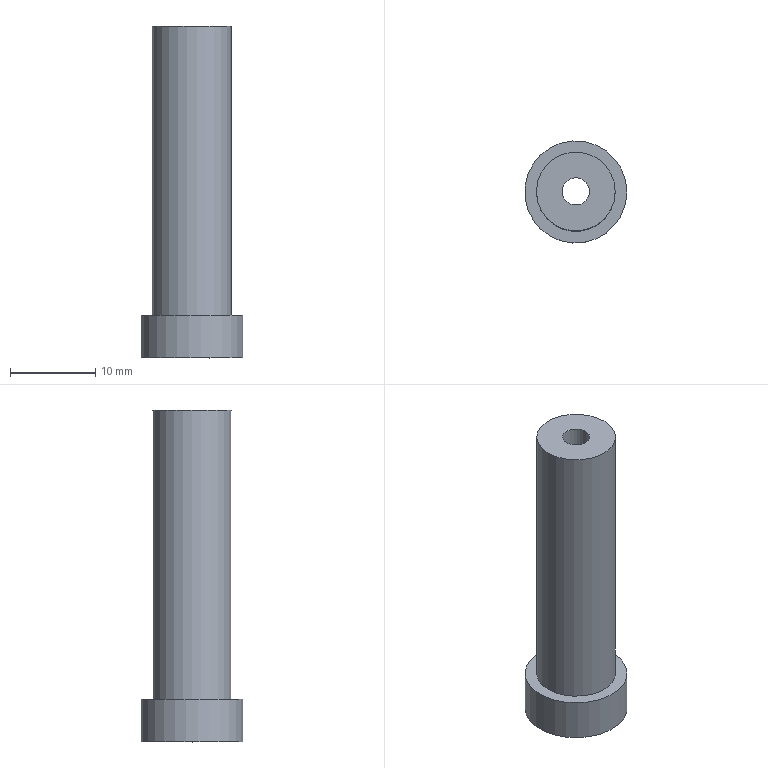Part | NX | features solid 2 | 1 solid | 8 faces | box 12 x 12 x 39 mm | volume 2338 mm3 | cylinder 4 | plane 4 | commonest cylinder face diameters 3.2 x1 4.2 x1 9.26 x1 12 x1
STEP:
#1=CARTESIAN_POINT('',(3190.896,-906.707,862.716));
#2=VERTEX_POINT('',#1);
#3=CARTESIAN_POINT('',(3186.266,-906.707,862.716));
#4=DIRECTION('',(0.,0.,1.));
#5=DIRECTION('',(1.,0.,0.));
#6=AXIS2_PLACEMENT_3D('',#3,#4,#5);
#7=CIRCLE('',#6,4.63);
#8=EDGE_CURVE('',#2,#2,#7,.T.);
#9=ORIENTED_EDGE('',*,*,#8,.F.);
#10=EDGE_LOOP('',(#9));
#11=FACE_BOUND('',#10,.T.);
#12=CARTESIAN_POINT('',(3190.896,-906.707,828.716));
#13=VERTEX_POINT('',#12);
#14=CARTESIAN_POINT('',(3186.266,-906.707,828.716));
#15=DIRECTION('',(0.,0.,1.));
#16=DIRECTION('',(1.,0.,0.));
#17=AXIS2_PLACEMENT_3D('',#14,#15,#16);
#18=CIRCLE('',#17,4.63);
#19=EDGE_CURVE('',#13,#13,#18,.T.);
#20=ORIENTED_EDGE('',*,*,#19,.T.);
#21=EDGE_LOOP('',(#20));
#22=FACE_BOUND('',#21,.T.);
#23=CARTESIAN_POINT('',(3186.266,-906.707,817.716));
#24=DIRECTION('',(0.,0.,1.));
#25=DIRECTION('',(1.,0.,0.));
#26=AXIS2_PLACEMENT_3D('',#23,#24,#25);
#27=CYLINDRICAL_SURFACE('',#26,4.63);
#28=ADVANCED_FACE('',(#11,#22),#27,.T.);
#29=CARTESIAN_POINT('',(3184.666,-906.707,858.716));
#30=VERTEX_POINT('',#29);
#31=CARTESIAN_POINT('',(3186.266,-906.707,858.716));
#32=DIRECTION('',(0.,0.,1.));
#33=DIRECTION('',(1.,0.,0.));
#34=AXIS2_PLACEMENT_3D('',#31,#32,#33);
#35=CIRCLE('',#34,1.6);
#36=EDGE_CURVE('',#30,#30,#35,.F.);
#37=ORIENTED_EDGE('',*,*,#36,.F.);
#38=EDGE_LOOP('',(#37));
#39=FACE_BOUND('',#38,.T.);
#40=CARTESIAN_POINT('',(3184.166,-906.707,858.716));
#41=VERTEX_POINT('',#40);
#42=CARTESIAN_POINT('',(3186.266,-906.707,858.716));
#43=DIRECTION('',(0.,0.,1.));
#44=DIRECTION('',(1.,0.,0.));
#45=AXIS2_PLACEMENT_3D('',#42,#43,#44);
#46=CIRCLE('',#45,2.1);
#47=EDGE_CURVE('',#41,#41,#46,.T.);
#48=ORIENTED_EDGE('',*,*,#47,.F.);
#49=EDGE_LOOP('',(#48));
#50=FACE_BOUND('',#49,.T.);
#51=CARTESIAN_POINT('',(3186.266,-906.707,858.716));
#52=DIRECTION('',(0.,0.,1.));
#53=DIRECTION('',(1.,0.,0.));
#54=AXIS2_PLACEMENT_3D('',#51,#52,#53);
#55=PLANE('',#54);
#56=ADVANCED_FACE('',(#39,#50),#55,.F.);
#57=CARTESIAN_POINT('',(3184.666,-906.707,862.716));
#58=VERTEX_POINT('',#57);
#59=CARTESIAN_POINT('',(3186.266,-906.707,862.716));
#60=DIRECTION('',(0.,0.,1.));
#61=DIRECTION('',(1.,0.,0.));
#62=AXIS2_PLACEMENT_3D('',#59,#60,#61);
#63=CIRCLE('',#62,1.6);
#64=EDGE_CURVE('',#58,#58,#63,.T.);
#65=ORIENTED_EDGE('',*,*,#64,.F.);
#66=EDGE_LOOP('',(#65));
#67=FACE_BOUND('',#66,.T.);
#68=ORIENTED_EDGE('',*,*,#8,.T.);
#69=EDGE_LOOP('',(#68));
#70=FACE_BOUND('',#69,.T.);
#71=CARTESIAN_POINT('',(3186.266,-906.707,862.716));
#72=DIRECTION('',(0.,0.,1.));
#73=DIRECTION('',(1.,0.,0.));
#74=AXIS2_PLACEMENT_3D('',#71,#72,#73);
#75=PLANE('',#74);
#76=ADVANCED_FACE('',(#67,#70),#75,.T.);
#77=CARTESIAN_POINT('',(3184.666,-906.707,867.216));
#78=DIRECTION('',(0.,0.,-1.));
#79=VECTOR('',#78,1000.);
#80=LINE('',#77,#79);
#81=EDGE_CURVE('',#58,#30,#80,.T.);
#82=ORIENTED_EDGE('',*,*,#81,.T.);
#83=ORIENTED_EDGE('',*,*,#36,.T.);
#84=ORIENTED_EDGE('',*,*,#81,.F.);
#85=ORIENTED_EDGE('',*,*,#64,.T.);
#86=EDGE_LOOP('',(#82,#83,#84,#85));
#87=FACE_BOUND('',#86,.T.);
#88=CARTESIAN_POINT('',(3186.266,-906.707,867.216));
#89=DIRECTION('',(0.,0.,-1.));
#90=DIRECTION('',(-1.,0.,0.));
#91=AXIS2_PLACEMENT_3D('',#88,#89,#90);
#92=CYLINDRICAL_SURFACE('',#91,1.6);
#93=ADVANCED_FACE('',(#87),#92,.F.);
#94=ORIENTED_EDGE('',*,*,#47,.T.);
#95=CARTESIAN_POINT('',(3184.166,-906.707,823.716));
#96=VERTEX_POINT('',#95);
#97=CARTESIAN_POINT('',(3184.166,-906.707,867.216));
#98=DIRECTION('',(0.,0.,-1.));
#99=VECTOR('',#98,1000.);
#100=LINE('',#97,#99);
#101=EDGE_CURVE('',#41,#96,#100,.T.);
#102=ORIENTED_EDGE('',*,*,#101,.T.);
#103=CARTESIAN_POINT('',(3186.266,-906.707,823.716));
#104=DIRECTION('',(0.,0.,-1.));
#105=DIRECTION('',(-1.,0.,0.));
#106=AXIS2_PLACEMENT_3D('',#103,#104,#105);
#107=CIRCLE('',#106,2.1);
#108=EDGE_CURVE('',#96,#96,#107,.F.);
#109=ORIENTED_EDGE('',*,*,#108,.F.);
#110=ORIENTED_EDGE('',*,*,#101,.F.);
#111=EDGE_LOOP('',(#94,#102,#109,#110));
#112=FACE_BOUND('',#111,.T.);
#113=CARTESIAN_POINT('',(3186.266,-906.707,867.216));
#114=DIRECTION('',(0.,0.,-1.));
#115=DIRECTION('',(-1.,0.,0.));
#116=AXIS2_PLACEMENT_3D('',#113,#114,#115);
#117=CYLINDRICAL_SURFACE('',#116,2.1);
#118=ADVANCED_FACE('',(#112),#117,.F.);
#119=ORIENTED_EDGE('',*,*,#108,.T.);
#120=EDGE_LOOP('',(#119));
#121=FACE_BOUND('',#120,.T.);
#122=CARTESIAN_POINT('',(3192.266,-906.707,823.716));
#123=VERTEX_POINT('',#122);
#124=CARTESIAN_POINT('',(3186.266,-906.707,823.716));
#125=DIRECTION('',(0.,0.,1.));
#126=DIRECTION('',(1.,0.,0.));
#127=AXIS2_PLACEMENT_3D('',#124,#125,#126);
#128=CIRCLE('',#127,6.);
#129=EDGE_CURVE('',#123,#123,#128,.T.);
#130=ORIENTED_EDGE('',*,*,#129,.F.);
#131=EDGE_LOOP('',(#130));
#132=FACE_BOUND('',#131,.T.);
#133=CARTESIAN_POINT('',(3186.266,-906.707,823.716));
#134=DIRECTION('',(0.,0.,-1.));
#135=DIRECTION('',(0.0349,0.9994,0.));
#136=AXIS2_PLACEMENT_3D('',#133,#134,#135);
#137=PLANE('',#136);
#138=ADVANCED_FACE('',(#121,#132),#137,.T.);
#139=ORIENTED_EDGE('',*,*,#19,.F.);
#140=EDGE_LOOP('',(#139));
#141=FACE_BOUND('',#140,.T.);
#142=CARTESIAN_POINT('',(3192.266,-906.707,828.716));
#143=VERTEX_POINT('',#142);
#144=CARTESIAN_POINT('',(3186.266,-906.707,828.716));
#145=DIRECTION('',(0.,0.,-1.));
#146=DIRECTION('',(1.,0.,0.));
#147=AXIS2_PLACEMENT_3D('',#144,#145,#146);
#148=CIRCLE('',#147,6.);
#149=EDGE_CURVE('',#143,#143,#148,.T.);
#150=ORIENTED_EDGE('',*,*,#149,.F.);
#151=EDGE_LOOP('',(#150));
#152=FACE_BOUND('',#151,.T.);
#153=CARTESIAN_POINT('',(3186.266,-906.707,828.716));
#154=DIRECTION('',(0.,0.,1.));
#155=DIRECTION('',(1.,0.,0.));
#156=AXIS2_PLACEMENT_3D('',#153,#154,#155);
#157=PLANE('',#156);
#158=ADVANCED_FACE('',(#141,#152),#157,.T.);
#159=ORIENTED_EDGE('',*,*,#149,.T.);
#160=EDGE_LOOP('',(#159));
#161=FACE_BOUND('',#160,.T.);
#162=ORIENTED_EDGE('',*,*,#129,.T.);
#163=EDGE_LOOP('',(#162));
#164=FACE_BOUND('',#163,.T.);
#165=CARTESIAN_POINT('',(3186.266,-906.707,823.716));
#166=DIRECTION('',(0.,0.,1.));
#167=DIRECTION('',(1.,0.,0.));
#168=AXIS2_PLACEMENT_3D('',#165,#166,#167);
#169=CYLINDRICAL_SURFACE('',#168,6.);
#170=ADVANCED_FACE('',(#161,#164),#169,.T.);
#171=CLOSED_SHELL('',(#28,#56,#76,#93,#118,#138,#158,#170));
#172=MANIFOLD_SOLID_BREP('',#171);
#173=(LENGTH_UNIT()NAMED_UNIT(*)SI_UNIT(.MILLI.,.METRE.));
#174=UNCERTAINTY_MEASURE_WITH_UNIT(LENGTH_MEASURE(0.00001),#173,'','');
#175=(NAMED_UNIT(*)PLANE_ANGLE_UNIT()SI_UNIT($,.RADIAN.));
#176=(NAMED_UNIT(*)SI_UNIT($,.STERADIAN.)SOLID_ANGLE_UNIT());
#177=(GEOMETRIC_REPRESENTATION_CONTEXT(3)GLOBAL_UNCERTAINTY_ASSIGNED_CONTEXT((#174))GLOBAL_UNIT_ASSIGNED_CONTEXT((#173,#175,#176))REPRESENTATION_CONTEXT('',''));
#178=ADVANCED_BREP_SHAPE_REPRESENTATION('',(#172),#177);